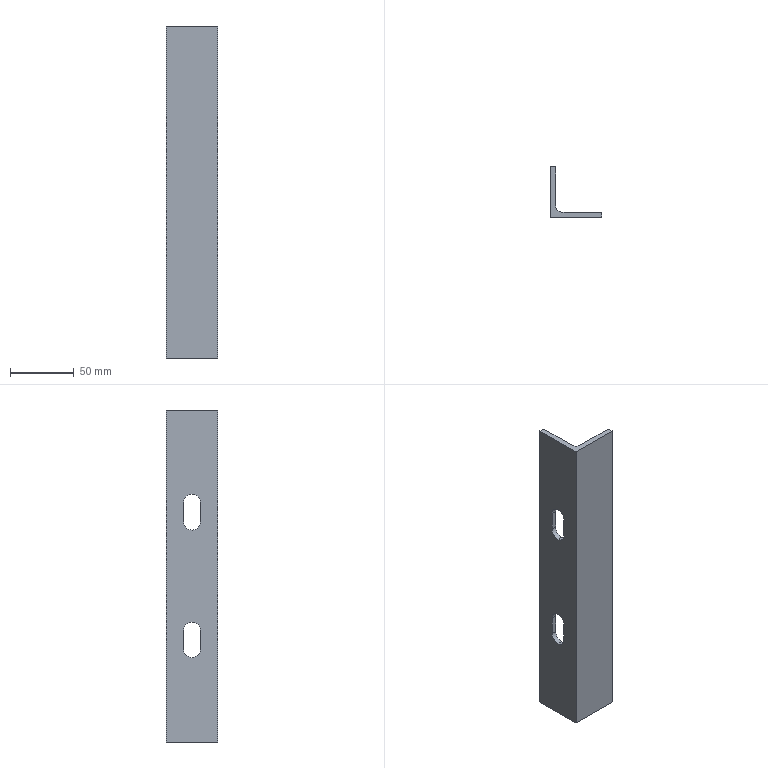Part | SolidWorks | features BaseBody 1 | 1 solid | 21 faces | box 40 x 40 x 260 mm | volume 77615 mm3 | plane 12 | cylinder 9 | commonest cylinder face diameters 13 x6 2.667 x2 10 x1
STEP:
#1=CARTESIAN_POINT('',(-11.3,31.3,66.));
#2=VERTEX_POINT('',#1);
#3=CARTESIAN_POINT('',(-11.3,37.8,72.5));
#4=VERTEX_POINT('',#3);
#5=CARTESIAN_POINT('',(-11.3,31.3,72.5));
#6=DIRECTION('',(1.,0.,0.));
#7=DIRECTION('',(0.,0.,-1.));
#8=AXIS2_PLACEMENT_3D('',#5,#6,#7);
#9=CIRCLE('',#8,6.5);
#10=EDGE_CURVE('',#2,#4,#9,.T.);
#11=ORIENTED_EDGE('',*,*,#10,.F.);
#12=CARTESIAN_POINT('',(-7.3,31.3,66.));
#13=VERTEX_POINT('',#12);
#14=CARTESIAN_POINT('',(-11.3,31.3,66.));
#15=DIRECTION('',(1.,0.,0.));
#16=VECTOR('',#15,1000.);
#17=LINE('',#14,#16);
#18=EDGE_CURVE('',#2,#13,#17,.T.);
#19=ORIENTED_EDGE('',*,*,#18,.T.);
#20=CARTESIAN_POINT('',(-7.3,37.8,72.5));
#21=VERTEX_POINT('',#20);
#22=CARTESIAN_POINT('',(-7.3,31.3,72.5));
#23=DIRECTION('',(-1.,0.,0.));
#24=DIRECTION('',(0.,0.,-1.));
#25=AXIS2_PLACEMENT_3D('',#22,#23,#24);
#26=CIRCLE('',#25,6.5);
#27=EDGE_CURVE('',#21,#13,#26,.T.);
#28=ORIENTED_EDGE('',*,*,#27,.F.);
#29=CARTESIAN_POINT('',(-11.3,37.8,72.5));
#30=DIRECTION('',(-1.,0.,0.));
#31=VECTOR('',#30,1000.);
#32=LINE('',#29,#31);
#33=EDGE_CURVE('',#21,#4,#32,.T.);
#34=ORIENTED_EDGE('',*,*,#33,.T.);
#35=EDGE_LOOP('',(#11,#19,#28,#34));
#36=FACE_OUTER_BOUND('',#35,.T.);
#37=CARTESIAN_POINT('',(-11.3,31.3,72.5));
#38=DIRECTION('',(1.,0.,0.));
#39=DIRECTION('',(0.,0.,-1.));
#40=AXIS2_PLACEMENT_3D('',#37,#38,#39);
#41=CYLINDRICAL_SURFACE('',#40,6.5);
#42=ADVANCED_FACE('',(#36),#41,.F.);
#43=CARTESIAN_POINT('',(-11.3,31.3,166.));
#44=VERTEX_POINT('',#43);
#45=CARTESIAN_POINT('',(-11.3,37.8,172.5));
#46=VERTEX_POINT('',#45);
#47=CARTESIAN_POINT('',(-11.3,31.3,172.5));
#48=DIRECTION('',(1.,0.,0.));
#49=DIRECTION('',(0.,0.,-1.));
#50=AXIS2_PLACEMENT_3D('',#47,#48,#49);
#51=CIRCLE('',#50,6.5);
#52=EDGE_CURVE('',#44,#46,#51,.T.);
#53=ORIENTED_EDGE('',*,*,#52,.F.);
#54=CARTESIAN_POINT('',(-7.3,31.3,166.));
#55=VERTEX_POINT('',#54);
#56=CARTESIAN_POINT('',(-11.3,31.3,166.));
#57=DIRECTION('',(1.,0.,0.));
#58=VECTOR('',#57,1000.);
#59=LINE('',#56,#58);
#60=EDGE_CURVE('',#44,#55,#59,.T.);
#61=ORIENTED_EDGE('',*,*,#60,.T.);
#62=CARTESIAN_POINT('',(-7.3,37.8,172.5));
#63=VERTEX_POINT('',#62);
#64=CARTESIAN_POINT('',(-7.3,31.3,172.5));
#65=DIRECTION('',(-1.,0.,0.));
#66=DIRECTION('',(0.,0.,-1.));
#67=AXIS2_PLACEMENT_3D('',#64,#65,#66);
#68=CIRCLE('',#67,6.5);
#69=EDGE_CURVE('',#63,#55,#68,.T.);
#70=ORIENTED_EDGE('',*,*,#69,.F.);
#71=CARTESIAN_POINT('',(-11.3,37.8,172.5));
#72=DIRECTION('',(-1.,0.,0.));
#73=VECTOR('',#72,1000.);
#74=LINE('',#71,#73);
#75=EDGE_CURVE('',#63,#46,#74,.T.);
#76=ORIENTED_EDGE('',*,*,#75,.T.);
#77=EDGE_LOOP('',(#53,#61,#70,#76));
#78=FACE_OUTER_BOUND('',#77,.T.);
#79=CARTESIAN_POINT('',(-11.3,31.3,172.5));
#80=DIRECTION('',(1.,0.,0.));
#81=DIRECTION('',(0.,0.,-1.));
#82=AXIS2_PLACEMENT_3D('',#79,#80,#81);
#83=CYLINDRICAL_SURFACE('',#82,6.5);
#84=ADVANCED_FACE('',(#78),#83,.F.);
#85=CARTESIAN_POINT('',(-11.3,11.3,0.));
#86=VERTEX_POINT('',#85);
#87=CARTESIAN_POINT('',(28.7,11.3,0.));
#88=VERTEX_POINT('',#87);
#89=CARTESIAN_POINT('',(28.7,11.3,0.));
#90=DIRECTION('',(1.,0.,0.));
#91=VECTOR('',#90,1000.);
#92=LINE('',#89,#91);
#93=EDGE_CURVE('',#86,#88,#92,.T.);
#94=ORIENTED_EDGE('',*,*,#93,.T.);
#95=CARTESIAN_POINT('',(28.7,11.3,260.));
#96=VERTEX_POINT('',#95);
#97=CARTESIAN_POINT('',(28.7,11.3,0.));
#98=DIRECTION('',(0.,0.,1.));
#99=VECTOR('',#98,1000.);
#100=LINE('',#97,#99);
#101=EDGE_CURVE('',#88,#96,#100,.T.);
#102=ORIENTED_EDGE('',*,*,#101,.T.);
#103=CARTESIAN_POINT('',(-11.3,11.3,260.));
#104=VERTEX_POINT('',#103);
#105=CARTESIAN_POINT('',(28.7,11.3,260.));
#106=DIRECTION('',(-1.,0.,0.));
#107=VECTOR('',#106,1000.);
#108=LINE('',#105,#107);
#109=EDGE_CURVE('',#96,#104,#108,.T.);
#110=ORIENTED_EDGE('',*,*,#109,.T.);
#111=CARTESIAN_POINT('',(-11.3,11.3,0.));
#112=DIRECTION('',(0.,0.,-1.));
#113=VECTOR('',#112,1000.);
#114=LINE('',#111,#113);
#115=EDGE_CURVE('',#104,#86,#114,.T.);
#116=ORIENTED_EDGE('',*,*,#115,.T.);
#117=EDGE_LOOP('',(#94,#102,#110,#116));
#118=FACE_OUTER_BOUND('',#117,.T.);
#119=CARTESIAN_POINT('',(28.7,11.3,0.));
#120=DIRECTION('',(0.,-1.,0.));
#121=DIRECTION('',(1.,0.,0.));
#122=AXIS2_PLACEMENT_3D('',#119,#120,#121);
#123=PLANE('',#122);
#124=ADVANCED_FACE('',(#118),#123,.T.);
#125=CARTESIAN_POINT('',(28.7,13.967,0.));
#126=VERTEX_POINT('',#125);
#127=CARTESIAN_POINT('',(28.7,13.967,0.));
#128=DIRECTION('',(0.,1.,0.));
#129=VECTOR('',#128,1000.);
#130=LINE('',#127,#129);
#131=EDGE_CURVE('',#88,#126,#130,.T.);
#132=ORIENTED_EDGE('',*,*,#131,.T.);
#133=CARTESIAN_POINT('',(28.7,13.967,260.));
#134=VERTEX_POINT('',#133);
#135=CARTESIAN_POINT('',(28.7,13.967,0.));
#136=DIRECTION('',(0.,0.,1.));
#137=VECTOR('',#136,1000.);
#138=LINE('',#135,#137);
#139=EDGE_CURVE('',#126,#134,#138,.T.);
#140=ORIENTED_EDGE('',*,*,#139,.T.);
#141=CARTESIAN_POINT('',(28.7,13.967,260.));
#142=DIRECTION('',(0.,-1.,0.));
#143=VECTOR('',#142,1000.);
#144=LINE('',#141,#143);
#145=EDGE_CURVE('',#134,#96,#144,.T.);
#146=ORIENTED_EDGE('',*,*,#145,.T.);
#147=ORIENTED_EDGE('',*,*,#101,.F.);
#148=EDGE_LOOP('',(#132,#140,#146,#147));
#149=FACE_OUTER_BOUND('',#148,.T.);
#150=CARTESIAN_POINT('',(28.7,13.967,0.));
#151=DIRECTION('',(1.,0.,0.));
#152=DIRECTION('',(0.,1.,0.));
#153=AXIS2_PLACEMENT_3D('',#150,#151,#152);
#154=PLANE('',#153);
#155=ADVANCED_FACE('',(#149),#154,.T.);
#156=CARTESIAN_POINT('',(-8.633,51.3,0.));
#157=VERTEX_POINT('',#156);
#158=CARTESIAN_POINT('',(-11.3,51.3,0.));
#159=VERTEX_POINT('',#158);
#160=CARTESIAN_POINT('',(8.7,51.3,0.));
#161=DIRECTION('',(-1.,0.,0.));
#162=VECTOR('',#161,1000.);
#163=LINE('',#160,#162);
#164=EDGE_CURVE('',#157,#159,#163,.T.);
#165=ORIENTED_EDGE('',*,*,#164,.F.);
#166=CARTESIAN_POINT('',(-7.3,49.967,0.));
#167=VERTEX_POINT('',#166);
#168=CARTESIAN_POINT('',(-8.633,49.967,0.));
#169=DIRECTION('',(0.,0.,1.));
#170=DIRECTION('',(1.,0.,0.));
#171=AXIS2_PLACEMENT_3D('',#168,#169,#170);
#172=CIRCLE('',#171,1.333);
#173=EDGE_CURVE('',#167,#157,#172,.T.);
#174=ORIENTED_EDGE('',*,*,#173,.F.);
#175=CARTESIAN_POINT('',(-7.3,20.3,0.));
#176=VERTEX_POINT('',#175);
#177=CARTESIAN_POINT('',(-7.3,31.3,0.));
#178=DIRECTION('',(0.,1.,0.));
#179=VECTOR('',#178,1000.);
#180=LINE('',#177,#179);
#181=EDGE_CURVE('',#176,#167,#180,.T.);
#182=ORIENTED_EDGE('',*,*,#181,.F.);
#183=CARTESIAN_POINT('',(-2.3,15.3,0.));
#184=VERTEX_POINT('',#183);
#185=CARTESIAN_POINT('',(-2.3,20.3,0.));
#186=DIRECTION('',(0.,0.,-1.));
#187=DIRECTION('',(1.,0.,0.));
#188=AXIS2_PLACEMENT_3D('',#185,#186,#187);
#189=CIRCLE('',#188,5.);
#190=EDGE_CURVE('',#184,#176,#189,.T.);
#191=ORIENTED_EDGE('',*,*,#190,.F.);
#192=CARTESIAN_POINT('',(27.367,15.3,0.));
#193=VERTEX_POINT('',#192);
#194=CARTESIAN_POINT('',(8.7,15.3,0.));
#195=DIRECTION('',(-1.,0.,0.));
#196=VECTOR('',#195,1000.);
#197=LINE('',#194,#196);
#198=EDGE_CURVE('',#193,#184,#197,.T.);
#199=ORIENTED_EDGE('',*,*,#198,.F.);
#200=CARTESIAN_POINT('',(27.367,13.967,0.));
#201=DIRECTION('',(0.,0.,1.));
#202=DIRECTION('',(1.,0.,0.));
#203=AXIS2_PLACEMENT_3D('',#200,#201,#202);
#204=CIRCLE('',#203,1.333);
#205=EDGE_CURVE('',#126,#193,#204,.T.);
#206=ORIENTED_EDGE('',*,*,#205,.F.);
#207=ORIENTED_EDGE('',*,*,#131,.F.);
#208=ORIENTED_EDGE('',*,*,#93,.F.);
#209=CARTESIAN_POINT('',(-11.3,31.3,0.));
#210=DIRECTION('',(0.,-1.,0.));
#211=VECTOR('',#210,1000.);
#212=LINE('',#209,#211);
#213=EDGE_CURVE('',#159,#86,#212,.T.);
#214=ORIENTED_EDGE('',*,*,#213,.F.);
#215=EDGE_LOOP('',(#165,#174,#182,#191,#199,#206,#207,#208,#214));
#216=FACE_OUTER_BOUND('',#215,.T.);
#217=CARTESIAN_POINT('',(8.7,31.3,0.));
#218=DIRECTION('',(0.,0.,1.));
#219=DIRECTION('',(1.,0.,0.));
#220=AXIS2_PLACEMENT_3D('',#217,#218,#219);
#221=PLANE('',#220);
#222=ADVANCED_FACE('',(#216),#221,.F.);
#223=CARTESIAN_POINT('',(-11.3,24.8,72.5));
#224=VERTEX_POINT('',#223);
#225=CARTESIAN_POINT('',(-11.3,31.3,72.5));
#226=DIRECTION('',(1.,0.,0.));
#227=DIRECTION('',(0.,0.,-1.));
#228=AXIS2_PLACEMENT_3D('',#225,#226,#227);
#229=CIRCLE('',#228,6.5);
#230=EDGE_CURVE('',#224,#2,#229,.T.);
#231=ORIENTED_EDGE('',*,*,#230,.T.);
#232=ORIENTED_EDGE('',*,*,#10,.T.);
#233=CARTESIAN_POINT('',(-11.3,37.8,87.5));
#234=VERTEX_POINT('',#233);
#235=CARTESIAN_POINT('',(-11.3,37.8,0.));
#236=DIRECTION('',(0.,0.,1.));
#237=VECTOR('',#236,1000.);
#238=LINE('',#235,#237);
#239=EDGE_CURVE('',#4,#234,#238,.T.);
#240=ORIENTED_EDGE('',*,*,#239,.T.);
#241=CARTESIAN_POINT('',(-11.3,24.8,87.5));
#242=VERTEX_POINT('',#241);
#243=CARTESIAN_POINT('',(-11.3,31.3,87.5));
#244=DIRECTION('',(1.,0.,0.));
#245=DIRECTION('',(0.,0.,-1.));
#246=AXIS2_PLACEMENT_3D('',#243,#244,#245);
#247=CIRCLE('',#246,6.5);
#248=EDGE_CURVE('',#234,#242,#247,.T.);
#249=ORIENTED_EDGE('',*,*,#248,.T.);
#250=CARTESIAN_POINT('',(-11.3,24.8,0.));
#251=DIRECTION('',(0.,0.,-1.));
#252=VECTOR('',#251,1000.);
#253=LINE('',#250,#252);
#254=EDGE_CURVE('',#242,#224,#253,.T.);
#255=ORIENTED_EDGE('',*,*,#254,.T.);
#256=EDGE_LOOP('',(#231,#232,#240,#249,#255));
#257=FACE_BOUND('',#256,.T.);
#258=CARTESIAN_POINT('',(-11.3,24.8,172.5));
#259=VERTEX_POINT('',#258);
#260=CARTESIAN_POINT('',(-11.3,31.3,172.5));
#261=DIRECTION('',(1.,0.,0.));
#262=DIRECTION('',(0.,0.,-1.));
#263=AXIS2_PLACEMENT_3D('',#260,#261,#262);
#264=CIRCLE('',#263,6.5);
#265=EDGE_CURVE('',#259,#44,#264,.T.);
#266=ORIENTED_EDGE('',*,*,#265,.T.);
#267=ORIENTED_EDGE('',*,*,#52,.T.);
#268=CARTESIAN_POINT('',(-11.3,37.8,187.5));
#269=VERTEX_POINT('',#268);
#270=CARTESIAN_POINT('',(-11.3,37.8,0.));
#271=DIRECTION('',(0.,0.,1.));
#272=VECTOR('',#271,1000.);
#273=LINE('',#270,#272);
#274=EDGE_CURVE('',#46,#269,#273,.T.);
#275=ORIENTED_EDGE('',*,*,#274,.T.);
#276=CARTESIAN_POINT('',(-11.3,24.8,187.5));
#277=VERTEX_POINT('',#276);
#278=CARTESIAN_POINT('',(-11.3,31.3,187.5));
#279=DIRECTION('',(1.,0.,0.));
#280=DIRECTION('',(0.,0.,-1.));
#281=AXIS2_PLACEMENT_3D('',#278,#279,#280);
#282=CIRCLE('',#281,6.5);
#283=EDGE_CURVE('',#269,#277,#282,.T.);
#284=ORIENTED_EDGE('',*,*,#283,.T.);
#285=CARTESIAN_POINT('',(-11.3,24.8,0.));
#286=DIRECTION('',(0.,0.,-1.));
#287=VECTOR('',#286,1000.);
#288=LINE('',#285,#287);
#289=EDGE_CURVE('',#277,#259,#288,.T.);
#290=ORIENTED_EDGE('',*,*,#289,.T.);
#291=EDGE_LOOP('',(#266,#267,#275,#284,#290));
#292=FACE_BOUND('',#291,.T.);
#293=ORIENTED_EDGE('',*,*,#213,.T.);
#294=ORIENTED_EDGE('',*,*,#115,.F.);
#295=CARTESIAN_POINT('',(-11.3,51.3,260.));
#296=VERTEX_POINT('',#295);
#297=CARTESIAN_POINT('',(-11.3,11.3,260.));
#298=DIRECTION('',(0.,1.,0.));
#299=VECTOR('',#298,1000.);
#300=LINE('',#297,#299);
#301=EDGE_CURVE('',#104,#296,#300,.T.);
#302=ORIENTED_EDGE('',*,*,#301,.T.);
#303=CARTESIAN_POINT('',(-11.3,51.3,0.));
#304=DIRECTION('',(0.,0.,-1.));
#305=VECTOR('',#304,1000.);
#306=LINE('',#303,#305);
#307=EDGE_CURVE('',#296,#159,#306,.T.);
#308=ORIENTED_EDGE('',*,*,#307,.T.);
#309=EDGE_LOOP('',(#293,#294,#302,#308));
#310=FACE_OUTER_BOUND('',#309,.T.);
#311=CARTESIAN_POINT('',(-11.3,11.3,0.));
#312=DIRECTION('',(-1.,0.,0.));
#313=DIRECTION('',(0.,-1.,0.));
#314=AXIS2_PLACEMENT_3D('',#311,#312,#313);
#315=PLANE('',#314);
#316=ADVANCED_FACE('',(#257,#292,#310),#315,.T.);
#317=CARTESIAN_POINT('',(-7.3,49.967,260.));
#318=VERTEX_POINT('',#317);
#319=CARTESIAN_POINT('',(-8.633,51.3,260.));
#320=VERTEX_POINT('',#319);
#321=CARTESIAN_POINT('',(-8.633,49.967,260.));
#322=DIRECTION('',(0.,0.,1.));
#323=DIRECTION('',(1.,0.,0.));
#324=AXIS2_PLACEMENT_3D('',#321,#322,#323);
#325=CIRCLE('',#324,1.333);
#326=EDGE_CURVE('',#318,#320,#325,.T.);
#327=ORIENTED_EDGE('',*,*,#326,.T.);
#328=CARTESIAN_POINT('',(8.7,51.3,260.));
#329=DIRECTION('',(-1.,0.,0.));
#330=VECTOR('',#329,1000.);
#331=LINE('',#328,#330);
#332=EDGE_CURVE('',#320,#296,#331,.T.);
#333=ORIENTED_EDGE('',*,*,#332,.T.);
#334=ORIENTED_EDGE('',*,*,#301,.F.);
#335=ORIENTED_EDGE('',*,*,#109,.F.);
#336=ORIENTED_EDGE('',*,*,#145,.F.);
#337=CARTESIAN_POINT('',(27.367,15.3,260.));
#338=VERTEX_POINT('',#337);
#339=CARTESIAN_POINT('',(27.367,13.967,260.));
#340=DIRECTION('',(0.,0.,1.));
#341=DIRECTION('',(1.,0.,0.));
#342=AXIS2_PLACEMENT_3D('',#339,#340,#341);
#343=CIRCLE('',#342,1.333);
#344=EDGE_CURVE('',#134,#338,#343,.T.);
#345=ORIENTED_EDGE('',*,*,#344,.T.);
#346=CARTESIAN_POINT('',(-2.3,15.3,260.));
#347=VERTEX_POINT('',#346);
#348=CARTESIAN_POINT('',(8.7,15.3,260.));
#349=DIRECTION('',(-1.,0.,0.));
#350=VECTOR('',#349,1000.);
#351=LINE('',#348,#350);
#352=EDGE_CURVE('',#338,#347,#351,.T.);
#353=ORIENTED_EDGE('',*,*,#352,.T.);
#354=CARTESIAN_POINT('',(-7.3,20.3,260.));
#355=VERTEX_POINT('',#354);
#356=CARTESIAN_POINT('',(-2.3,20.3,260.));
#357=DIRECTION('',(0.,0.,-1.));
#358=DIRECTION('',(1.,0.,0.));
#359=AXIS2_PLACEMENT_3D('',#356,#357,#358);
#360=CIRCLE('',#359,5.);
#361=EDGE_CURVE('',#347,#355,#360,.T.);
#362=ORIENTED_EDGE('',*,*,#361,.T.);
#363=CARTESIAN_POINT('',(-7.3,31.3,260.));
#364=DIRECTION('',(0.,1.,0.));
#365=VECTOR('',#364,1000.);
#366=LINE('',#363,#365);
#367=EDGE_CURVE('',#355,#318,#366,.T.);
#368=ORIENTED_EDGE('',*,*,#367,.T.);
#369=EDGE_LOOP('',(#327,#333,#334,#335,#336,#345,#353,#362,#368));
#370=FACE_OUTER_BOUND('',#369,.T.);
#371=CARTESIAN_POINT('',(8.7,31.3,260.));
#372=DIRECTION('',(0.,0.,1.));
#373=DIRECTION('',(1.,0.,0.));
#374=AXIS2_PLACEMENT_3D('',#371,#372,#373);
#375=PLANE('',#374);
#376=ADVANCED_FACE('',(#370),#375,.T.);
#377=ORIENTED_EDGE('',*,*,#205,.T.);
#378=CARTESIAN_POINT('',(27.367,15.3,0.));
#379=DIRECTION('',(0.,0.,1.));
#380=VECTOR('',#379,1000.);
#381=LINE('',#378,#380);
#382=EDGE_CURVE('',#193,#338,#381,.T.);
#383=ORIENTED_EDGE('',*,*,#382,.T.);
#384=ORIENTED_EDGE('',*,*,#344,.F.);
#385=ORIENTED_EDGE('',*,*,#139,.F.);
#386=EDGE_LOOP('',(#377,#383,#384,#385));
#387=FACE_OUTER_BOUND('',#386,.T.);
#388=CARTESIAN_POINT('',(27.367,13.967,0.));
#389=DIRECTION('',(0.,0.,1.));
#390=DIRECTION('',(1.,0.,0.));
#391=AXIS2_PLACEMENT_3D('',#388,#389,#390);
#392=CYLINDRICAL_SURFACE('',#391,1.333);
#393=ADVANCED_FACE('',(#387),#392,.T.);
#394=ORIENTED_EDGE('',*,*,#164,.T.);
#395=ORIENTED_EDGE('',*,*,#307,.F.);
#396=ORIENTED_EDGE('',*,*,#332,.F.);
#397=CARTESIAN_POINT('',(-8.633,51.3,0.));
#398=DIRECTION('',(0.,0.,-1.));
#399=VECTOR('',#398,1000.);
#400=LINE('',#397,#399);
#401=EDGE_CURVE('',#320,#157,#400,.T.);
#402=ORIENTED_EDGE('',*,*,#401,.T.);
#403=EDGE_LOOP('',(#394,#395,#396,#402));
#404=FACE_OUTER_BOUND('',#403,.T.);
#405=CARTESIAN_POINT('',(-11.3,51.3,0.));
#406=DIRECTION('',(0.,1.,0.));
#407=DIRECTION('',(0.,0.,1.));
#408=AXIS2_PLACEMENT_3D('',#405,#406,#407);
#409=PLANE('',#408);
#410=ADVANCED_FACE('',(#404),#409,.T.);
#411=ORIENTED_EDGE('',*,*,#173,.T.);
#412=ORIENTED_EDGE('',*,*,#401,.F.);
#413=ORIENTED_EDGE('',*,*,#326,.F.);
#414=CARTESIAN_POINT('',(-7.3,49.967,0.));
#415=DIRECTION('',(0.,0.,-1.));
#416=VECTOR('',#415,1000.);
#417=LINE('',#414,#416);
#418=EDGE_CURVE('',#318,#167,#417,.T.);
#419=ORIENTED_EDGE('',*,*,#418,.T.);
#420=EDGE_LOOP('',(#411,#412,#413,#419));
#421=FACE_OUTER_BOUND('',#420,.T.);
#422=CARTESIAN_POINT('',(-8.633,49.967,0.));
#423=DIRECTION('',(0.,0.,1.));
#424=DIRECTION('',(1.,0.,0.));
#425=AXIS2_PLACEMENT_3D('',#422,#423,#424);
#426=CYLINDRICAL_SURFACE('',#425,1.333);
#427=ADVANCED_FACE('',(#421),#426,.T.);
#428=ORIENTED_EDGE('',*,*,#27,.T.);
#429=CARTESIAN_POINT('',(-7.3,24.8,72.5));
#430=VERTEX_POINT('',#429);
#431=CARTESIAN_POINT('',(-7.3,31.3,72.5));
#432=DIRECTION('',(-1.,0.,0.));
#433=DIRECTION('',(0.,0.,-1.));
#434=AXIS2_PLACEMENT_3D('',#431,#432,#433);
#435=CIRCLE('',#434,6.5);
#436=EDGE_CURVE('',#13,#430,#435,.T.);
#437=ORIENTED_EDGE('',*,*,#436,.T.);
#438=CARTESIAN_POINT('',(-7.3,24.8,87.5));
#439=VERTEX_POINT('',#438);
#440=CARTESIAN_POINT('',(-7.3,24.8,0.));
#441=DIRECTION('',(0.,0.,1.));
#442=VECTOR('',#441,1000.);
#443=LINE('',#440,#442);
#444=EDGE_CURVE('',#430,#439,#443,.T.);
#445=ORIENTED_EDGE('',*,*,#444,.T.);
#446=CARTESIAN_POINT('',(-7.3,37.8,87.5));
#447=VERTEX_POINT('',#446);
#448=CARTESIAN_POINT('',(-7.3,31.3,87.5));
#449=DIRECTION('',(-1.,0.,0.));
#450=DIRECTION('',(0.,0.,-1.));
#451=AXIS2_PLACEMENT_3D('',#448,#449,#450);
#452=CIRCLE('',#451,6.5);
#453=EDGE_CURVE('',#439,#447,#452,.T.);
#454=ORIENTED_EDGE('',*,*,#453,.T.);
#455=CARTESIAN_POINT('',(-7.3,37.8,0.));
#456=DIRECTION('',(0.,0.,-1.));
#457=VECTOR('',#456,1000.);
#458=LINE('',#455,#457);
#459=EDGE_CURVE('',#447,#21,#458,.T.);
#460=ORIENTED_EDGE('',*,*,#459,.T.);
#461=EDGE_LOOP('',(#428,#437,#445,#454,#460));
#462=FACE_BOUND('',#461,.T.);
#463=ORIENTED_EDGE('',*,*,#69,.T.);
#464=CARTESIAN_POINT('',(-7.3,24.8,172.5));
#465=VERTEX_POINT('',#464);
#466=CARTESIAN_POINT('',(-7.3,31.3,172.5));
#467=DIRECTION('',(-1.,0.,0.));
#468=DIRECTION('',(0.,0.,-1.));
#469=AXIS2_PLACEMENT_3D('',#466,#467,#468);
#470=CIRCLE('',#469,6.5);
#471=EDGE_CURVE('',#55,#465,#470,.T.);
#472=ORIENTED_EDGE('',*,*,#471,.T.);
#473=CARTESIAN_POINT('',(-7.3,24.8,187.5));
#474=VERTEX_POINT('',#473);
#475=CARTESIAN_POINT('',(-7.3,24.8,0.));
#476=DIRECTION('',(0.,0.,1.));
#477=VECTOR('',#476,1000.);
#478=LINE('',#475,#477);
#479=EDGE_CURVE('',#465,#474,#478,.T.);
#480=ORIENTED_EDGE('',*,*,#479,.T.);
#481=CARTESIAN_POINT('',(-7.3,37.8,187.5));
#482=VERTEX_POINT('',#481);
#483=CARTESIAN_POINT('',(-7.3,31.3,187.5));
#484=DIRECTION('',(-1.,0.,0.));
#485=DIRECTION('',(0.,0.,-1.));
#486=AXIS2_PLACEMENT_3D('',#483,#484,#485);
#487=CIRCLE('',#486,6.5);
#488=EDGE_CURVE('',#474,#482,#487,.T.);
#489=ORIENTED_EDGE('',*,*,#488,.T.);
#490=CARTESIAN_POINT('',(-7.3,37.8,0.));
#491=DIRECTION('',(0.,0.,-1.));
#492=VECTOR('',#491,1000.);
#493=LINE('',#490,#492);
#494=EDGE_CURVE('',#482,#63,#493,.T.);
#495=ORIENTED_EDGE('',*,*,#494,.T.);
#496=EDGE_LOOP('',(#463,#472,#480,#489,#495));
#497=FACE_BOUND('',#496,.T.);
#498=ORIENTED_EDGE('',*,*,#181,.T.);
#499=ORIENTED_EDGE('',*,*,#418,.F.);
#500=ORIENTED_EDGE('',*,*,#367,.F.);
#501=CARTESIAN_POINT('',(-7.3,20.3,0.));
#502=DIRECTION('',(0.,0.,-1.));
#503=VECTOR('',#502,1000.);
#504=LINE('',#501,#503);
#505=EDGE_CURVE('',#355,#176,#504,.T.);
#506=ORIENTED_EDGE('',*,*,#505,.T.);
#507=EDGE_LOOP('',(#498,#499,#500,#506));
#508=FACE_OUTER_BOUND('',#507,.T.);
#509=CARTESIAN_POINT('',(-7.3,49.967,0.));
#510=DIRECTION('',(1.,0.,0.));
#511=DIRECTION('',(0.,1.,0.));
#512=AXIS2_PLACEMENT_3D('',#509,#510,#511);
#513=PLANE('',#512);
#514=ADVANCED_FACE('',(#462,#497,#508),#513,.T.);
#515=CARTESIAN_POINT('',(-2.3,15.3,0.));
#516=DIRECTION('',(0.,0.,1.));
#517=VECTOR('',#516,1000.);
#518=LINE('',#515,#517);
#519=EDGE_CURVE('',#184,#347,#518,.T.);
#520=ORIENTED_EDGE('',*,*,#519,.F.);
#521=ORIENTED_EDGE('',*,*,#190,.T.);
#522=ORIENTED_EDGE('',*,*,#505,.F.);
#523=ORIENTED_EDGE('',*,*,#361,.F.);
#524=EDGE_LOOP('',(#520,#521,#522,#523));
#525=FACE_OUTER_BOUND('',#524,.T.);
#526=CARTESIAN_POINT('',(-2.3,20.3,0.));
#527=DIRECTION('',(0.,0.,1.));
#528=DIRECTION('',(1.,0.,0.));
#529=AXIS2_PLACEMENT_3D('',#526,#527,#528);
#530=CYLINDRICAL_SURFACE('',#529,5.);
#531=ADVANCED_FACE('',(#525),#530,.F.);
#532=ORIENTED_EDGE('',*,*,#198,.T.);
#533=ORIENTED_EDGE('',*,*,#519,.T.);
#534=ORIENTED_EDGE('',*,*,#352,.F.);
#535=ORIENTED_EDGE('',*,*,#382,.F.);
#536=EDGE_LOOP('',(#532,#533,#534,#535));
#537=FACE_OUTER_BOUND('',#536,.T.);
#538=CARTESIAN_POINT('',(-2.3,15.3,0.));
#539=DIRECTION('',(0.,1.,0.));
#540=DIRECTION('',(-1.,0.,0.));
#541=AXIS2_PLACEMENT_3D('',#538,#539,#540);
#542=PLANE('',#541);
#543=ADVANCED_FACE('',(#537),#542,.T.);
#544=CARTESIAN_POINT('',(-11.3,37.8,87.5));
#545=DIRECTION('',(1.,0.,0.));
#546=VECTOR('',#545,1000.);
#547=LINE('',#544,#546);
#548=EDGE_CURVE('',#234,#447,#547,.T.);
#549=ORIENTED_EDGE('',*,*,#548,.F.);
#550=ORIENTED_EDGE('',*,*,#239,.F.);
#551=ORIENTED_EDGE('',*,*,#33,.F.);
#552=ORIENTED_EDGE('',*,*,#459,.F.);
#553=EDGE_LOOP('',(#549,#550,#551,#552));
#554=FACE_OUTER_BOUND('',#553,.T.);
#555=CARTESIAN_POINT('',(-11.3,37.8,72.5));
#556=DIRECTION('',(0.,1.,0.));
#557=DIRECTION('',(0.,0.,1.));
#558=AXIS2_PLACEMENT_3D('',#555,#556,#557);
#559=PLANE('',#558);
#560=ADVANCED_FACE('',(#554),#559,.F.);
#561=ORIENTED_EDGE('',*,*,#18,.F.);
#562=ORIENTED_EDGE('',*,*,#230,.F.);
#563=CARTESIAN_POINT('',(-11.3,24.8,72.5));
#564=DIRECTION('',(-1.,0.,0.));
#565=VECTOR('',#564,1000.);
#566=LINE('',#563,#565);
#567=EDGE_CURVE('',#430,#224,#566,.T.);
#568=ORIENTED_EDGE('',*,*,#567,.F.);
#569=ORIENTED_EDGE('',*,*,#436,.F.);
#570=EDGE_LOOP('',(#561,#562,#568,#569));
#571=FACE_OUTER_BOUND('',#570,.T.);
#572=CARTESIAN_POINT('',(-11.3,31.3,72.5));
#573=DIRECTION('',(1.,0.,0.));
#574=DIRECTION('',(0.,0.,-1.));
#575=AXIS2_PLACEMENT_3D('',#572,#573,#574);
#576=CYLINDRICAL_SURFACE('',#575,6.5);
#577=ADVANCED_FACE('',(#571),#576,.F.);
#578=ORIENTED_EDGE('',*,*,#567,.T.);
#579=ORIENTED_EDGE('',*,*,#254,.F.);
#580=CARTESIAN_POINT('',(-11.3,24.8,87.5));
#581=DIRECTION('',(-1.,0.,0.));
#582=VECTOR('',#581,1000.);
#583=LINE('',#580,#582);
#584=EDGE_CURVE('',#439,#242,#583,.T.);
#585=ORIENTED_EDGE('',*,*,#584,.F.);
#586=ORIENTED_EDGE('',*,*,#444,.F.);
#587=EDGE_LOOP('',(#578,#579,#585,#586));
#588=FACE_OUTER_BOUND('',#587,.T.);
#589=CARTESIAN_POINT('',(-11.3,24.8,87.5));
#590=DIRECTION('',(0.,-1.,0.));
#591=DIRECTION('',(0.,0.,-1.));
#592=AXIS2_PLACEMENT_3D('',#589,#590,#591);
#593=PLANE('',#592);
#594=ADVANCED_FACE('',(#588),#593,.F.);
#595=ORIENTED_EDGE('',*,*,#584,.T.);
#596=ORIENTED_EDGE('',*,*,#248,.F.);
#597=ORIENTED_EDGE('',*,*,#548,.T.);
#598=ORIENTED_EDGE('',*,*,#453,.F.);
#599=EDGE_LOOP('',(#595,#596,#597,#598));
#600=FACE_OUTER_BOUND('',#599,.T.);
#601=CARTESIAN_POINT('',(-11.3,31.3,87.5));
#602=DIRECTION('',(1.,0.,0.));
#603=DIRECTION('',(0.,0.,-1.));
#604=AXIS2_PLACEMENT_3D('',#601,#602,#603);
#605=CYLINDRICAL_SURFACE('',#604,6.5);
#606=ADVANCED_FACE('',(#600),#605,.F.);
#607=CARTESIAN_POINT('',(-11.3,37.8,187.5));
#608=DIRECTION('',(1.,0.,0.));
#609=VECTOR('',#608,1000.);
#610=LINE('',#607,#609);
#611=EDGE_CURVE('',#269,#482,#610,.T.);
#612=ORIENTED_EDGE('',*,*,#611,.F.);
#613=ORIENTED_EDGE('',*,*,#274,.F.);
#614=ORIENTED_EDGE('',*,*,#75,.F.);
#615=ORIENTED_EDGE('',*,*,#494,.F.);
#616=EDGE_LOOP('',(#612,#613,#614,#615));
#617=FACE_OUTER_BOUND('',#616,.T.);
#618=CARTESIAN_POINT('',(-11.3,37.8,172.5));
#619=DIRECTION('',(0.,1.,0.));
#620=DIRECTION('',(0.,0.,1.));
#621=AXIS2_PLACEMENT_3D('',#618,#619,#620);
#622=PLANE('',#621);
#623=ADVANCED_FACE('',(#617),#622,.F.);
#624=ORIENTED_EDGE('',*,*,#60,.F.);
#625=ORIENTED_EDGE('',*,*,#265,.F.);
#626=CARTESIAN_POINT('',(-11.3,24.8,172.5));
#627=DIRECTION('',(-1.,0.,0.));
#628=VECTOR('',#627,1000.);
#629=LINE('',#626,#628);
#630=EDGE_CURVE('',#465,#259,#629,.T.);
#631=ORIENTED_EDGE('',*,*,#630,.F.);
#632=ORIENTED_EDGE('',*,*,#471,.F.);
#633=EDGE_LOOP('',(#624,#625,#631,#632));
#634=FACE_OUTER_BOUND('',#633,.T.);
#635=CARTESIAN_POINT('',(-11.3,31.3,172.5));
#636=DIRECTION('',(1.,0.,0.));
#637=DIRECTION('',(0.,0.,-1.));
#638=AXIS2_PLACEMENT_3D('',#635,#636,#637);
#639=CYLINDRICAL_SURFACE('',#638,6.5);
#640=ADVANCED_FACE('',(#634),#639,.F.);
#641=ORIENTED_EDGE('',*,*,#630,.T.);
#642=ORIENTED_EDGE('',*,*,#289,.F.);
#643=CARTESIAN_POINT('',(-11.3,24.8,187.5));
#644=DIRECTION('',(-1.,0.,0.));
#645=VECTOR('',#644,1000.);
#646=LINE('',#643,#645);
#647=EDGE_CURVE('',#474,#277,#646,.T.);
#648=ORIENTED_EDGE('',*,*,#647,.F.);
#649=ORIENTED_EDGE('',*,*,#479,.F.);
#650=EDGE_LOOP('',(#641,#642,#648,#649));
#651=FACE_OUTER_BOUND('',#650,.T.);
#652=CARTESIAN_POINT('',(-11.3,24.8,187.5));
#653=DIRECTION('',(0.,-1.,0.));
#654=DIRECTION('',(0.,0.,-1.));
#655=AXIS2_PLACEMENT_3D('',#652,#653,#654);
#656=PLANE('',#655);
#657=ADVANCED_FACE('',(#651),#656,.F.);
#658=ORIENTED_EDGE('',*,*,#647,.T.);
#659=ORIENTED_EDGE('',*,*,#283,.F.);
#660=ORIENTED_EDGE('',*,*,#611,.T.);
#661=ORIENTED_EDGE('',*,*,#488,.F.);
#662=EDGE_LOOP('',(#658,#659,#660,#661));
#663=FACE_OUTER_BOUND('',#662,.T.);
#664=CARTESIAN_POINT('',(-11.3,31.3,187.5));
#665=DIRECTION('',(1.,0.,0.));
#666=DIRECTION('',(0.,0.,-1.));
#667=AXIS2_PLACEMENT_3D('',#664,#665,#666);
#668=CYLINDRICAL_SURFACE('',#667,6.5);
#669=ADVANCED_FACE('',(#663),#668,.F.);
#670=CLOSED_SHELL('',(#42,#84,#124,#155,#222,#316,#376,#393,#410,#427,#514,#531,#543,#560,#577,#594,#606,#623,#640,#657,#669));
#671=MANIFOLD_SOLID_BREP('',#670);
#672=CARTESIAN_POINT('',(0.,0.,0.));
#673=DIRECTION('',(0.,0.,1.));
#674=DIRECTION('',(1.,0.,0.));
#675=AXIS2_PLACEMENT_3D('',#672,#673,#674);
#676=(LENGTH_UNIT()NAMED_UNIT(*)SI_UNIT(.MILLI.,.METRE.));
#677=UNCERTAINTY_MEASURE_WITH_UNIT(LENGTH_MEASURE(0.00001),#676,'','');
#678=(NAMED_UNIT(*)PLANE_ANGLE_UNIT()SI_UNIT($,.RADIAN.));
#679=(NAMED_UNIT(*)SI_UNIT($,.STERADIAN.)SOLID_ANGLE_UNIT());
#680=(GEOMETRIC_REPRESENTATION_CONTEXT(3)GLOBAL_UNCERTAINTY_ASSIGNED_CONTEXT((#677))GLOBAL_UNIT_ASSIGNED_CONTEXT((#676,#678,#679))REPRESENTATION_CONTEXT('',''));
#681=ADVANCED_BREP_SHAPE_REPRESENTATION('',(#671,#675),#680);